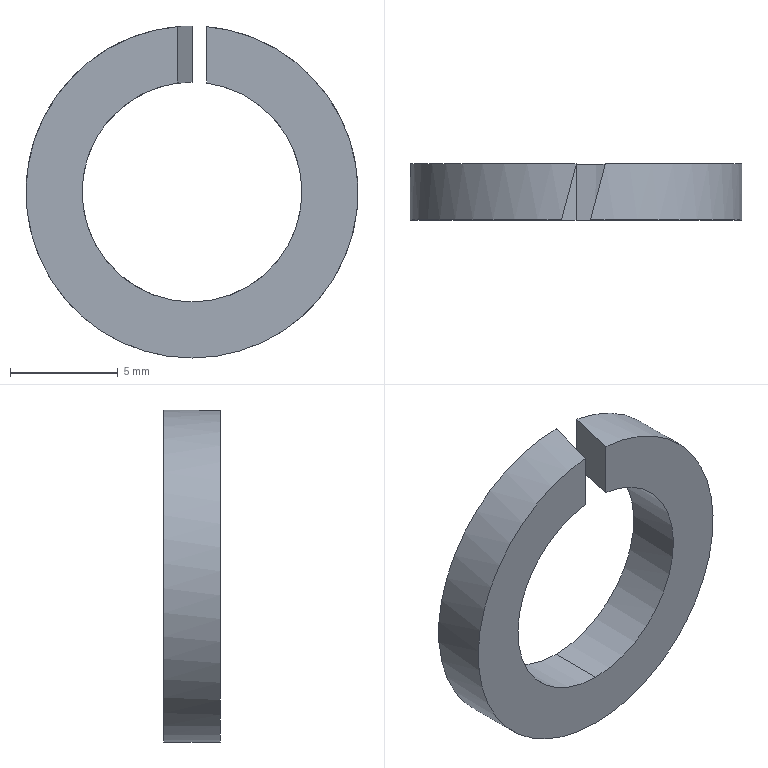Part | SolidWorks | features ICE 2, Extrusion 1 | 1 solid | 469 faces | box 15.4 x 2.6 x 15.4 mm | volume 262.555 mm3 | plane 328 | spline 135 | cylinder 6 | commonest cylinder face diameters 10.2 x3 15.4 x3